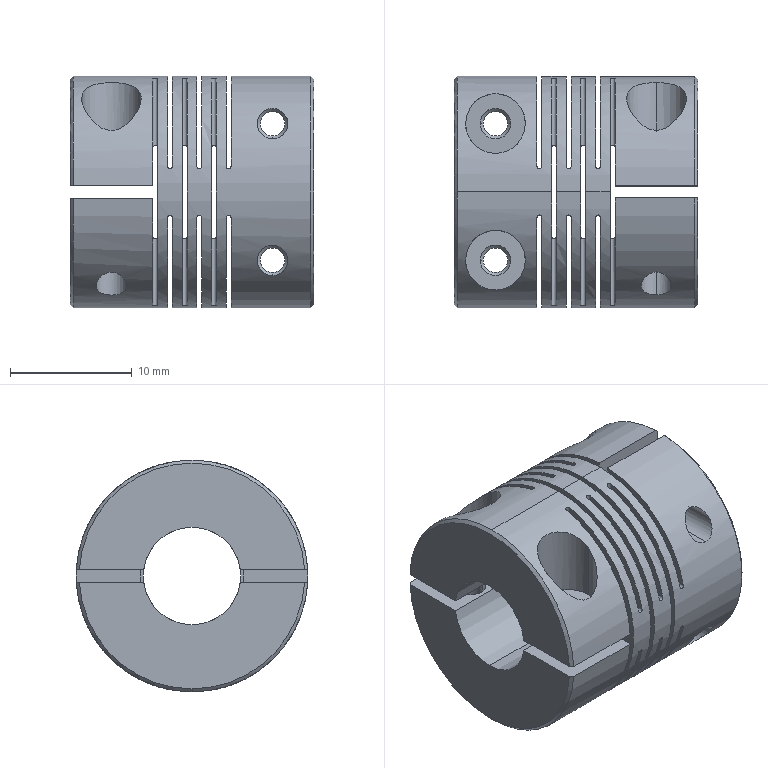Part | SolidWorks | features BaseBody 1 | 1 solid | 132 faces | box 20 x 19 x 19 mm | volume 3525 mm3 | cylinder 71 | plane 40 | cone 21 | commonest cylinder face diameters 0.4 x30 2.5 x16 2.013 x8 4.9 x8 8 x5 8.5 x2